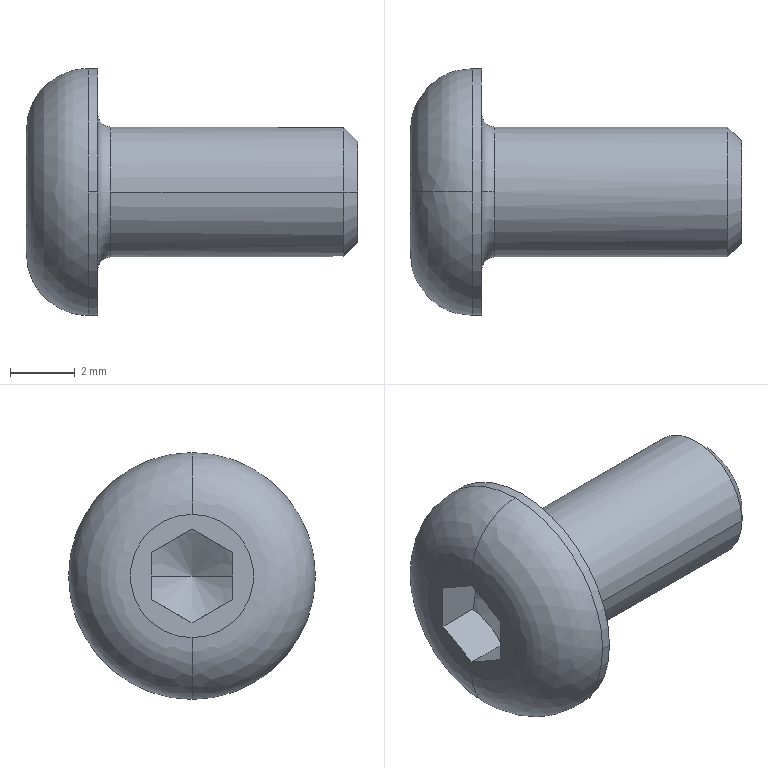Part | STEP file | ISO 7380-1 - M4 x 8 | 1 solid | 21 faces | box 10.2 x 7.6 x 7.6 mm | volume 174.472 mm3 | plane 9 | cylinder 4 | cone 4 | spline 2 | torus 2 | commonest cylinder face diameters 4 x2 7.6 x2